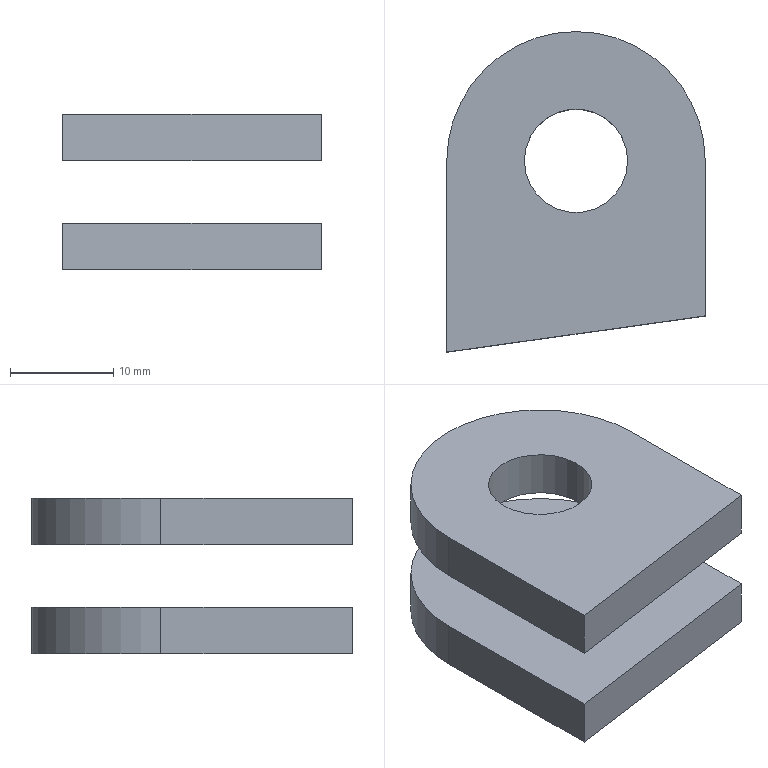Part | SolidWorks | features Extrusion 1, ICE 1 | 2 solids | 16 faces | box 25 x 31.014 x 15 mm | volume 5272 mm3 | plane 10 | cylinder 6 | commonest cylinder face diameters 10 x4 25 x2
STEP:
#1=CARTESIAN_POINT('',(5.,0.,4.5));
#2=VERTEX_POINT('',#1);
#3=CARTESIAN_POINT('',(-5.,0.,4.5));
#4=VERTEX_POINT('',#3);
#5=CARTESIAN_POINT('',(0.,0.,4.5));
#6=DIRECTION('',(0.,0.,-1.));
#7=DIRECTION('',(0.,1.,0.));
#8=AXIS2_PLACEMENT_3D('',#5,#6,#7);
#9=CIRCLE('',#8,5.);
#10=EDGE_CURVE('',#2,#4,#9,.T.);
#11=ORIENTED_EDGE('',*,*,#10,.F.);
#12=CARTESIAN_POINT('',(5.,0.,0.));
#13=VERTEX_POINT('',#12);
#14=CARTESIAN_POINT('',(5.,0.,15.));
#15=DIRECTION('',(0.,0.,-1.));
#16=VECTOR('',#15,1000.);
#17=LINE('',#14,#16);
#18=EDGE_CURVE('',#2,#13,#17,.T.);
#19=ORIENTED_EDGE('',*,*,#18,.T.);
#20=CARTESIAN_POINT('',(-5.,0.,0.));
#21=VERTEX_POINT('',#20);
#22=CARTESIAN_POINT('',(0.,0.,0.));
#23=DIRECTION('',(0.,0.,1.));
#24=DIRECTION('',(1.,0.,0.));
#25=AXIS2_PLACEMENT_3D('',#22,#23,#24);
#26=CIRCLE('',#25,5.);
#27=EDGE_CURVE('',#21,#13,#26,.T.);
#28=ORIENTED_EDGE('',*,*,#27,.F.);
#29=CARTESIAN_POINT('',(-5.,0.,15.));
#30=DIRECTION('',(0.,0.,-1.));
#31=VECTOR('',#30,1000.);
#32=LINE('',#29,#31);
#33=EDGE_CURVE('',#4,#21,#32,.T.);
#34=ORIENTED_EDGE('',*,*,#33,.F.);
#35=EDGE_LOOP('',(#11,#19,#28,#34));
#36=FACE_OUTER_BOUND('',#35,.T.);
#37=CARTESIAN_POINT('',(0.,0.,15.));
#38=DIRECTION('',(0.,0.,-1.));
#39=DIRECTION('',(-1.,0.,0.));
#40=AXIS2_PLACEMENT_3D('',#37,#38,#39);
#41=CYLINDRICAL_SURFACE('',#40,5.);
#42=ADVANCED_FACE('',(#36),#41,.F.);
#43=CARTESIAN_POINT('',(-12.5,0.,4.5));
#44=VERTEX_POINT('',#43);
#45=CARTESIAN_POINT('',(-12.5,0.,0.));
#46=VERTEX_POINT('',#45);
#47=CARTESIAN_POINT('',(-12.5,0.,15.));
#48=DIRECTION('',(0.,0.,-1.));
#49=VECTOR('',#48,1000.);
#50=LINE('',#47,#49);
#51=EDGE_CURVE('',#44,#46,#50,.T.);
#52=ORIENTED_EDGE('',*,*,#51,.F.);
#53=CARTESIAN_POINT('',(12.5,0.,4.5));
#54=VERTEX_POINT('',#53);
#55=CARTESIAN_POINT('',(0.,0.,4.5));
#56=DIRECTION('',(0.,0.,-1.));
#57=DIRECTION('',(0.,1.,0.));
#58=AXIS2_PLACEMENT_3D('',#55,#56,#57);
#59=CIRCLE('',#58,12.5);
#60=EDGE_CURVE('',#44,#54,#59,.T.);
#61=ORIENTED_EDGE('',*,*,#60,.T.);
#62=CARTESIAN_POINT('',(12.5,0.,0.));
#63=VERTEX_POINT('',#62);
#64=CARTESIAN_POINT('',(12.5,0.,15.));
#65=DIRECTION('',(0.,0.,-1.));
#66=VECTOR('',#65,1000.);
#67=LINE('',#64,#66);
#68=EDGE_CURVE('',#54,#63,#67,.T.);
#69=ORIENTED_EDGE('',*,*,#68,.T.);
#70=CARTESIAN_POINT('',(0.,0.,0.));
#71=DIRECTION('',(0.,0.,1.));
#72=DIRECTION('',(1.,0.,0.));
#73=AXIS2_PLACEMENT_3D('',#70,#71,#72);
#74=CIRCLE('',#73,12.5);
#75=EDGE_CURVE('',#63,#46,#74,.T.);
#76=ORIENTED_EDGE('',*,*,#75,.T.);
#77=EDGE_LOOP('',(#52,#61,#69,#76));
#78=FACE_OUTER_BOUND('',#77,.T.);
#79=CARTESIAN_POINT('',(0.,0.,15.));
#80=DIRECTION('',(0.,0.,-1.));
#81=DIRECTION('',(-1.,0.,0.));
#82=AXIS2_PLACEMENT_3D('',#79,#80,#81);
#83=CYLINDRICAL_SURFACE('',#82,12.5);
#84=ADVANCED_FACE('',(#78),#83,.T.);
#85=CARTESIAN_POINT('',(-12.5,-18.514,4.5));
#86=VERTEX_POINT('',#85);
#87=CARTESIAN_POINT('',(-12.5,-18.514,0.));
#88=VERTEX_POINT('',#87);
#89=CARTESIAN_POINT('',(-12.5,-18.514,15.));
#90=DIRECTION('',(0.,0.,-1.));
#91=VECTOR('',#90,1000.);
#92=LINE('',#89,#91);
#93=EDGE_CURVE('',#86,#88,#92,.T.);
#94=ORIENTED_EDGE('',*,*,#93,.F.);
#95=CARTESIAN_POINT('',(-12.5,57.491,4.5));
#96=DIRECTION('',(0.,1.,0.));
#97=VECTOR('',#96,1000.);
#98=LINE('',#95,#97);
#99=EDGE_CURVE('',#86,#44,#98,.T.);
#100=ORIENTED_EDGE('',*,*,#99,.T.);
#101=ORIENTED_EDGE('',*,*,#51,.T.);
#102=CARTESIAN_POINT('',(-12.5,0.,0.));
#103=DIRECTION('',(0.,-1.,0.));
#104=VECTOR('',#103,1000.);
#105=LINE('',#102,#104);
#106=EDGE_CURVE('',#46,#88,#105,.T.);
#107=ORIENTED_EDGE('',*,*,#106,.T.);
#108=EDGE_LOOP('',(#94,#100,#101,#107));
#109=FACE_OUTER_BOUND('',#108,.T.);
#110=CARTESIAN_POINT('',(-12.5,0.,15.));
#111=DIRECTION('',(1.,0.,0.));
#112=DIRECTION('',(0.,1.,0.));
#113=AXIS2_PLACEMENT_3D('',#110,#111,#112);
#114=PLANE('',#113);
#115=ADVANCED_FACE('',(#109),#114,.F.);
#116=CARTESIAN_POINT('',(12.5,-15.,4.5));
#117=VERTEX_POINT('',#116);
#118=CARTESIAN_POINT('',(2.309,-16.432,4.5));
#119=DIRECTION('',(0.9903,0.1392,0.));
#120=VECTOR('',#119,1000.);
#121=LINE('',#118,#120);
#122=EDGE_CURVE('',#86,#117,#121,.T.);
#123=ORIENTED_EDGE('',*,*,#122,.F.);
#124=ORIENTED_EDGE('',*,*,#93,.T.);
#125=CARTESIAN_POINT('',(12.5,-15.,0.));
#126=VERTEX_POINT('',#125);
#127=CARTESIAN_POINT('',(2.309,-16.432,0.));
#128=DIRECTION('',(-0.9903,-0.1392,0.));
#129=VECTOR('',#128,1000.);
#130=LINE('',#127,#129);
#131=EDGE_CURVE('',#126,#88,#130,.T.);
#132=ORIENTED_EDGE('',*,*,#131,.F.);
#133=CARTESIAN_POINT('',(12.5,-15.,15.));
#134=DIRECTION('',(0.,0.,-1.));
#135=VECTOR('',#134,1000.);
#136=LINE('',#133,#135);
#137=EDGE_CURVE('',#117,#126,#136,.T.);
#138=ORIENTED_EDGE('',*,*,#137,.F.);
#139=EDGE_LOOP('',(#123,#124,#132,#138));
#140=FACE_OUTER_BOUND('',#139,.T.);
#141=CARTESIAN_POINT('',(2.309,-16.432,15.));
#142=DIRECTION('',(0.1392,-0.9903,0.));
#143=DIRECTION('',(0.9903,0.1392,0.));
#144=AXIS2_PLACEMENT_3D('',#141,#142,#143);
#145=PLANE('',#144);
#146=ADVANCED_FACE('',(#140),#145,.T.);
#147=ORIENTED_EDGE('',*,*,#18,.F.);
#148=CARTESIAN_POINT('',(0.,0.,4.5));
#149=DIRECTION('',(0.,0.,-1.));
#150=DIRECTION('',(0.,1.,0.));
#151=AXIS2_PLACEMENT_3D('',#148,#149,#150);
#152=CIRCLE('',#151,5.);
#153=EDGE_CURVE('',#4,#2,#152,.T.);
#154=ORIENTED_EDGE('',*,*,#153,.F.);
#155=ORIENTED_EDGE('',*,*,#33,.T.);
#156=CARTESIAN_POINT('',(0.,0.,0.));
#157=DIRECTION('',(0.,0.,1.));
#158=DIRECTION('',(1.,0.,0.));
#159=AXIS2_PLACEMENT_3D('',#156,#157,#158);
#160=CIRCLE('',#159,5.);
#161=EDGE_CURVE('',#13,#21,#160,.T.);
#162=ORIENTED_EDGE('',*,*,#161,.F.);
#163=EDGE_LOOP('',(#147,#154,#155,#162));
#164=FACE_OUTER_BOUND('',#163,.T.);
#165=CARTESIAN_POINT('',(0.,0.,15.));
#166=DIRECTION('',(0.,0.,-1.));
#167=DIRECTION('',(-1.,0.,0.));
#168=AXIS2_PLACEMENT_3D('',#165,#166,#167);
#169=CYLINDRICAL_SURFACE('',#168,5.);
#170=ADVANCED_FACE('',(#164),#169,.F.);
#171=CARTESIAN_POINT('',(12.5,0.,4.5));
#172=DIRECTION('',(0.,1.,0.));
#173=VECTOR('',#172,1000.);
#174=LINE('',#171,#173);
#175=EDGE_CURVE('',#117,#54,#174,.T.);
#176=ORIENTED_EDGE('',*,*,#175,.F.);
#177=ORIENTED_EDGE('',*,*,#137,.T.);
#178=CARTESIAN_POINT('',(12.5,0.,0.));
#179=DIRECTION('',(0.,-1.,0.));
#180=VECTOR('',#179,1000.);
#181=LINE('',#178,#180);
#182=EDGE_CURVE('',#63,#126,#181,.T.);
#183=ORIENTED_EDGE('',*,*,#182,.F.);
#184=ORIENTED_EDGE('',*,*,#68,.F.);
#185=EDGE_LOOP('',(#176,#177,#183,#184));
#186=FACE_OUTER_BOUND('',#185,.T.);
#187=CARTESIAN_POINT('',(12.5,0.,15.));
#188=DIRECTION('',(1.,0.,0.));
#189=DIRECTION('',(0.,1.,0.));
#190=AXIS2_PLACEMENT_3D('',#187,#188,#189);
#191=PLANE('',#190);
#192=ADVANCED_FACE('',(#186),#191,.T.);
#193=ORIENTED_EDGE('',*,*,#27,.T.);
#194=ORIENTED_EDGE('',*,*,#161,.T.);
#195=EDGE_LOOP('',(#193,#194));
#196=FACE_BOUND('',#195,.T.);
#197=ORIENTED_EDGE('',*,*,#75,.F.);
#198=ORIENTED_EDGE('',*,*,#182,.T.);
#199=ORIENTED_EDGE('',*,*,#131,.T.);
#200=ORIENTED_EDGE('',*,*,#106,.F.);
#201=EDGE_LOOP('',(#197,#198,#199,#200));
#202=FACE_OUTER_BOUND('',#201,.T.);
#203=CARTESIAN_POINT('',(0.,0.,0.));
#204=DIRECTION('',(0.,0.,1.));
#205=DIRECTION('',(1.,0.,0.));
#206=AXIS2_PLACEMENT_3D('',#203,#204,#205);
#207=PLANE('',#206);
#208=ADVANCED_FACE('',(#196,#202),#207,.F.);
#209=ORIENTED_EDGE('',*,*,#153,.T.);
#210=ORIENTED_EDGE('',*,*,#10,.T.);
#211=EDGE_LOOP('',(#209,#210));
#212=FACE_BOUND('',#211,.T.);
#213=ORIENTED_EDGE('',*,*,#99,.F.);
#214=ORIENTED_EDGE('',*,*,#122,.T.);
#215=ORIENTED_EDGE('',*,*,#175,.T.);
#216=ORIENTED_EDGE('',*,*,#60,.F.);
#217=EDGE_LOOP('',(#213,#214,#215,#216));
#218=FACE_OUTER_BOUND('',#217,.T.);
#219=CARTESIAN_POINT('',(-12.5,57.491,4.5));
#220=DIRECTION('',(0.,0.,-1.));
#221=DIRECTION('',(0.,1.,0.));
#222=AXIS2_PLACEMENT_3D('',#219,#220,#221);
#223=PLANE('',#222);
#224=ADVANCED_FACE('',(#212,#218),#223,.F.);
#225=CLOSED_SHELL('',(#42,#84,#115,#146,#170,#192,#208,#224));
#226=MANIFOLD_SOLID_BREP('',#225);
#227=CARTESIAN_POINT('',(-5.,0.,15.));
#228=VERTEX_POINT('',#227);
#229=CARTESIAN_POINT('',(5.,0.,15.));
#230=VERTEX_POINT('',#229);
#231=CARTESIAN_POINT('',(0.,0.,15.));
#232=DIRECTION('',(0.,0.,1.));
#233=DIRECTION('',(1.,0.,0.));
#234=AXIS2_PLACEMENT_3D('',#231,#232,#233);
#235=CIRCLE('',#234,5.);
#236=EDGE_CURVE('',#228,#230,#235,.T.);
#237=ORIENTED_EDGE('',*,*,#236,.T.);
#238=CARTESIAN_POINT('',(5.,0.,10.5));
#239=VERTEX_POINT('',#238);
#240=CARTESIAN_POINT('',(5.,0.,15.));
#241=DIRECTION('',(0.,0.,-1.));
#242=VECTOR('',#241,1000.);
#243=LINE('',#240,#242);
#244=EDGE_CURVE('',#230,#239,#243,.T.);
#245=ORIENTED_EDGE('',*,*,#244,.T.);
#246=CARTESIAN_POINT('',(-5.,0.,10.5));
#247=VERTEX_POINT('',#246);
#248=CARTESIAN_POINT('',(0.,0.,10.5));
#249=DIRECTION('',(0.,0.,1.));
#250=DIRECTION('',(0.,-1.,0.));
#251=AXIS2_PLACEMENT_3D('',#248,#249,#250);
#252=CIRCLE('',#251,5.);
#253=EDGE_CURVE('',#247,#239,#252,.T.);
#254=ORIENTED_EDGE('',*,*,#253,.F.);
#255=CARTESIAN_POINT('',(-5.,0.,15.));
#256=DIRECTION('',(0.,0.,-1.));
#257=VECTOR('',#256,1000.);
#258=LINE('',#255,#257);
#259=EDGE_CURVE('',#228,#247,#258,.T.);
#260=ORIENTED_EDGE('',*,*,#259,.F.);
#261=EDGE_LOOP('',(#237,#245,#254,#260));
#262=FACE_OUTER_BOUND('',#261,.T.);
#263=CARTESIAN_POINT('',(0.,0.,15.));
#264=DIRECTION('',(0.,0.,-1.));
#265=DIRECTION('',(-1.,0.,0.));
#266=AXIS2_PLACEMENT_3D('',#263,#264,#265);
#267=CYLINDRICAL_SURFACE('',#266,5.);
#268=ADVANCED_FACE('',(#262),#267,.F.);
#269=ORIENTED_EDGE('',*,*,#244,.F.);
#270=CARTESIAN_POINT('',(0.,0.,15.));
#271=DIRECTION('',(0.,0.,1.));
#272=DIRECTION('',(1.,0.,0.));
#273=AXIS2_PLACEMENT_3D('',#270,#271,#272);
#274=CIRCLE('',#273,5.);
#275=EDGE_CURVE('',#230,#228,#274,.T.);
#276=ORIENTED_EDGE('',*,*,#275,.T.);
#277=ORIENTED_EDGE('',*,*,#259,.T.);
#278=CARTESIAN_POINT('',(0.,0.,10.5));
#279=DIRECTION('',(0.,0.,1.));
#280=DIRECTION('',(0.,-1.,0.));
#281=AXIS2_PLACEMENT_3D('',#278,#279,#280);
#282=CIRCLE('',#281,5.);
#283=EDGE_CURVE('',#239,#247,#282,.T.);
#284=ORIENTED_EDGE('',*,*,#283,.F.);
#285=EDGE_LOOP('',(#269,#276,#277,#284));
#286=FACE_OUTER_BOUND('',#285,.T.);
#287=CARTESIAN_POINT('',(0.,0.,15.));
#288=DIRECTION('',(0.,0.,-1.));
#289=DIRECTION('',(-1.,0.,0.));
#290=AXIS2_PLACEMENT_3D('',#287,#288,#289);
#291=CYLINDRICAL_SURFACE('',#290,5.);
#292=ADVANCED_FACE('',(#286),#291,.F.);
#293=ORIENTED_EDGE('',*,*,#236,.F.);
#294=ORIENTED_EDGE('',*,*,#275,.F.);
#295=EDGE_LOOP('',(#293,#294));
#296=FACE_BOUND('',#295,.T.);
#297=CARTESIAN_POINT('',(12.5,0.,15.));
#298=VERTEX_POINT('',#297);
#299=CARTESIAN_POINT('',(-12.5,0.,15.));
#300=VERTEX_POINT('',#299);
#301=CARTESIAN_POINT('',(0.,0.,15.));
#302=DIRECTION('',(0.,0.,1.));
#303=DIRECTION('',(1.,0.,0.));
#304=AXIS2_PLACEMENT_3D('',#301,#302,#303);
#305=CIRCLE('',#304,12.5);
#306=EDGE_CURVE('',#298,#300,#305,.T.);
#307=ORIENTED_EDGE('',*,*,#306,.T.);
#308=CARTESIAN_POINT('',(-12.5,-18.514,15.));
#309=VERTEX_POINT('',#308);
#310=CARTESIAN_POINT('',(-12.5,0.,15.));
#311=DIRECTION('',(0.,-1.,0.));
#312=VECTOR('',#311,1000.);
#313=LINE('',#310,#312);
#314=EDGE_CURVE('',#300,#309,#313,.T.);
#315=ORIENTED_EDGE('',*,*,#314,.T.);
#316=CARTESIAN_POINT('',(12.5,-15.,15.));
#317=VERTEX_POINT('',#316);
#318=CARTESIAN_POINT('',(2.309,-16.432,15.));
#319=DIRECTION('',(-0.9903,-0.1392,0.));
#320=VECTOR('',#319,1000.);
#321=LINE('',#318,#320);
#322=EDGE_CURVE('',#317,#309,#321,.T.);
#323=ORIENTED_EDGE('',*,*,#322,.F.);
#324=CARTESIAN_POINT('',(12.5,0.,15.));
#325=DIRECTION('',(0.,-1.,0.));
#326=VECTOR('',#325,1000.);
#327=LINE('',#324,#326);
#328=EDGE_CURVE('',#298,#317,#327,.T.);
#329=ORIENTED_EDGE('',*,*,#328,.F.);
#330=EDGE_LOOP('',(#307,#315,#323,#329));
#331=FACE_OUTER_BOUND('',#330,.T.);
#332=CARTESIAN_POINT('',(0.,0.,15.));
#333=DIRECTION('',(0.,0.,1.));
#334=DIRECTION('',(1.,0.,0.));
#335=AXIS2_PLACEMENT_3D('',#332,#333,#334);
#336=PLANE('',#335);
#337=ADVANCED_FACE('',(#296,#331),#336,.T.);
#338=CARTESIAN_POINT('',(12.5,0.,10.5));
#339=VERTEX_POINT('',#338);
#340=CARTESIAN_POINT('',(12.5,-15.,10.5));
#341=VERTEX_POINT('',#340);
#342=CARTESIAN_POINT('',(12.5,0.,10.5));
#343=DIRECTION('',(0.,-1.,0.));
#344=VECTOR('',#343,1000.);
#345=LINE('',#342,#344);
#346=EDGE_CURVE('',#339,#341,#345,.T.);
#347=ORIENTED_EDGE('',*,*,#346,.F.);
#348=CARTESIAN_POINT('',(12.5,0.,15.));
#349=DIRECTION('',(0.,0.,-1.));
#350=VECTOR('',#349,1000.);
#351=LINE('',#348,#350);
#352=EDGE_CURVE('',#298,#339,#351,.T.);
#353=ORIENTED_EDGE('',*,*,#352,.F.);
#354=ORIENTED_EDGE('',*,*,#328,.T.);
#355=CARTESIAN_POINT('',(12.5,-15.,15.));
#356=DIRECTION('',(0.,0.,-1.));
#357=VECTOR('',#356,1000.);
#358=LINE('',#355,#357);
#359=EDGE_CURVE('',#317,#341,#358,.T.);
#360=ORIENTED_EDGE('',*,*,#359,.T.);
#361=EDGE_LOOP('',(#347,#353,#354,#360));
#362=FACE_OUTER_BOUND('',#361,.T.);
#363=CARTESIAN_POINT('',(12.5,0.,15.));
#364=DIRECTION('',(1.,0.,0.));
#365=DIRECTION('',(0.,1.,0.));
#366=AXIS2_PLACEMENT_3D('',#363,#364,#365);
#367=PLANE('',#366);
#368=ADVANCED_FACE('',(#362),#367,.T.);
#369=CARTESIAN_POINT('',(-12.5,-18.514,10.5));
#370=VERTEX_POINT('',#369);
#371=CARTESIAN_POINT('',(2.309,-16.432,10.5));
#372=DIRECTION('',(-0.9903,-0.1392,0.));
#373=VECTOR('',#372,1000.);
#374=LINE('',#371,#373);
#375=EDGE_CURVE('',#341,#370,#374,.T.);
#376=ORIENTED_EDGE('',*,*,#375,.F.);
#377=ORIENTED_EDGE('',*,*,#359,.F.);
#378=ORIENTED_EDGE('',*,*,#322,.T.);
#379=CARTESIAN_POINT('',(-12.5,-18.514,15.));
#380=DIRECTION('',(0.,0.,-1.));
#381=VECTOR('',#380,1000.);
#382=LINE('',#379,#381);
#383=EDGE_CURVE('',#309,#370,#382,.T.);
#384=ORIENTED_EDGE('',*,*,#383,.T.);
#385=EDGE_LOOP('',(#376,#377,#378,#384));
#386=FACE_OUTER_BOUND('',#385,.T.);
#387=CARTESIAN_POINT('',(2.309,-16.432,15.));
#388=DIRECTION('',(0.1392,-0.9903,0.));
#389=DIRECTION('',(0.9903,0.1392,0.));
#390=AXIS2_PLACEMENT_3D('',#387,#388,#389);
#391=PLANE('',#390);
#392=ADVANCED_FACE('',(#386),#391,.T.);
#393=CARTESIAN_POINT('',(-12.5,0.,10.5));
#394=VERTEX_POINT('',#393);
#395=CARTESIAN_POINT('',(-12.5,0.,15.));
#396=DIRECTION('',(0.,0.,-1.));
#397=VECTOR('',#396,1000.);
#398=LINE('',#395,#397);
#399=EDGE_CURVE('',#300,#394,#398,.T.);
#400=ORIENTED_EDGE('',*,*,#399,.T.);
#401=CARTESIAN_POINT('',(-12.5,57.491,10.5));
#402=DIRECTION('',(0.,-1.,0.));
#403=VECTOR('',#402,1000.);
#404=LINE('',#401,#403);
#405=EDGE_CURVE('',#394,#370,#404,.T.);
#406=ORIENTED_EDGE('',*,*,#405,.T.);
#407=ORIENTED_EDGE('',*,*,#383,.F.);
#408=ORIENTED_EDGE('',*,*,#314,.F.);
#409=EDGE_LOOP('',(#400,#406,#407,#408));
#410=FACE_OUTER_BOUND('',#409,.T.);
#411=CARTESIAN_POINT('',(-12.5,0.,15.));
#412=DIRECTION('',(1.,0.,0.));
#413=DIRECTION('',(0.,1.,0.));
#414=AXIS2_PLACEMENT_3D('',#411,#412,#413);
#415=PLANE('',#414);
#416=ADVANCED_FACE('',(#410),#415,.F.);
#417=ORIENTED_EDGE('',*,*,#352,.T.);
#418=CARTESIAN_POINT('',(0.,0.,10.5));
#419=DIRECTION('',(0.,0.,1.));
#420=DIRECTION('',(0.,-1.,0.));
#421=AXIS2_PLACEMENT_3D('',#418,#419,#420);
#422=CIRCLE('',#421,12.5);
#423=EDGE_CURVE('',#339,#394,#422,.T.);
#424=ORIENTED_EDGE('',*,*,#423,.T.);
#425=ORIENTED_EDGE('',*,*,#399,.F.);
#426=ORIENTED_EDGE('',*,*,#306,.F.);
#427=EDGE_LOOP('',(#417,#424,#425,#426));
#428=FACE_OUTER_BOUND('',#427,.T.);
#429=CARTESIAN_POINT('',(0.,0.,15.));
#430=DIRECTION('',(0.,0.,-1.));
#431=DIRECTION('',(-1.,0.,0.));
#432=AXIS2_PLACEMENT_3D('',#429,#430,#431);
#433=CYLINDRICAL_SURFACE('',#432,12.5);
#434=ADVANCED_FACE('',(#428),#433,.T.);
#435=ORIENTED_EDGE('',*,*,#253,.T.);
#436=ORIENTED_EDGE('',*,*,#283,.T.);
#437=EDGE_LOOP('',(#435,#436));
#438=FACE_BOUND('',#437,.T.);
#439=ORIENTED_EDGE('',*,*,#346,.T.);
#440=ORIENTED_EDGE('',*,*,#375,.T.);
#441=ORIENTED_EDGE('',*,*,#405,.F.);
#442=ORIENTED_EDGE('',*,*,#423,.F.);
#443=EDGE_LOOP('',(#439,#440,#441,#442));
#444=FACE_OUTER_BOUND('',#443,.T.);
#445=CARTESIAN_POINT('',(-12.5,57.491,10.5));
#446=DIRECTION('',(0.,0.,1.));
#447=DIRECTION('',(0.,-1.,0.));
#448=AXIS2_PLACEMENT_3D('',#445,#446,#447);
#449=PLANE('',#448);
#450=ADVANCED_FACE('',(#438,#444),#449,.F.);
#451=CLOSED_SHELL('',(#268,#292,#337,#368,#392,#416,#434,#450));
#452=MANIFOLD_SOLID_BREP('',#451);
#453=CARTESIAN_POINT('',(0.,0.,0.));
#454=DIRECTION('',(0.,0.,1.));
#455=DIRECTION('',(1.,0.,0.));
#456=AXIS2_PLACEMENT_3D('',#453,#454,#455);
#457=(LENGTH_UNIT()NAMED_UNIT(*)SI_UNIT(.MILLI.,.METRE.));
#458=UNCERTAINTY_MEASURE_WITH_UNIT(LENGTH_MEASURE(0.00001),#457,'','');
#459=(NAMED_UNIT(*)PLANE_ANGLE_UNIT()SI_UNIT($,.RADIAN.));
#460=(NAMED_UNIT(*)SI_UNIT($,.STERADIAN.)SOLID_ANGLE_UNIT());
#461=(GEOMETRIC_REPRESENTATION_CONTEXT(3)GLOBAL_UNCERTAINTY_ASSIGNED_CONTEXT((#458))GLOBAL_UNIT_ASSIGNED_CONTEXT((#457,#459,#460))REPRESENTATION_CONTEXT('',''));
#462=ADVANCED_BREP_SHAPE_REPRESENTATION('',(#226,#452,#456),#461);